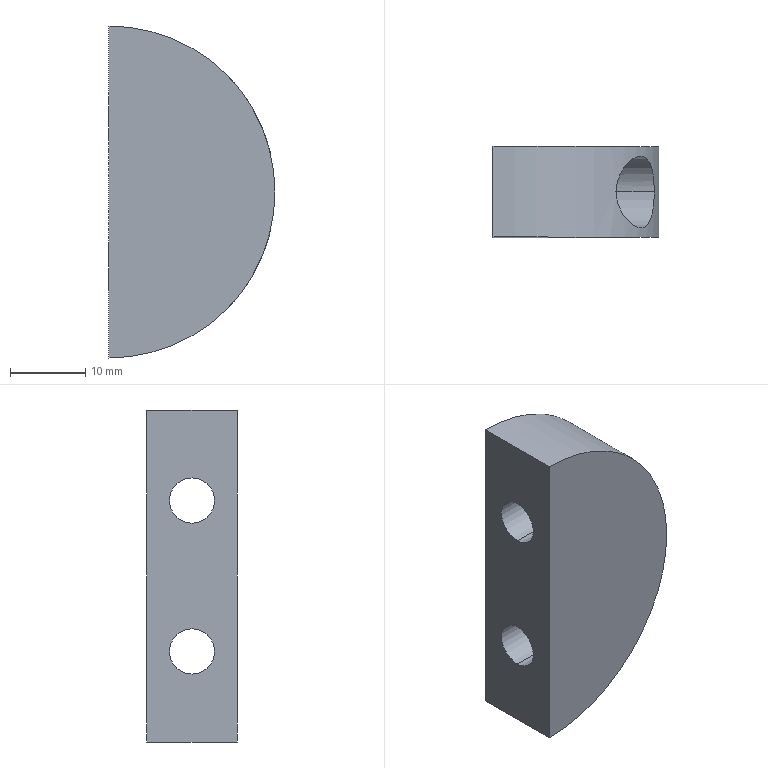Part | STEP file | OP10-147_seal side plate (2) | 1 solid | 14 faces | box 22 x 12 x 44 mm | volume 7394 mm3 | cylinder 9 | plane 5 | commonest cylinder face diameters 6 x4 9.5 x4 44 x1